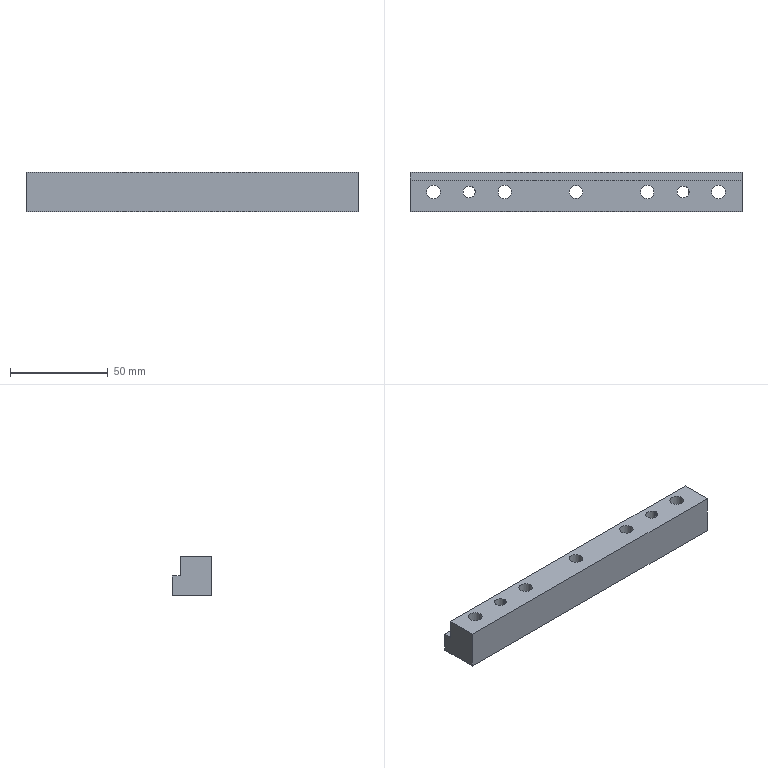Part | STEP file | 1 solid | 31 faces | box 170 x 20 x 20 mm | volume 54220 mm3 | cylinder 18 | plane 13 | commonest cylinder face diameters 1 x6 11 x5 6.8 x3 6.01 x2 7 x2